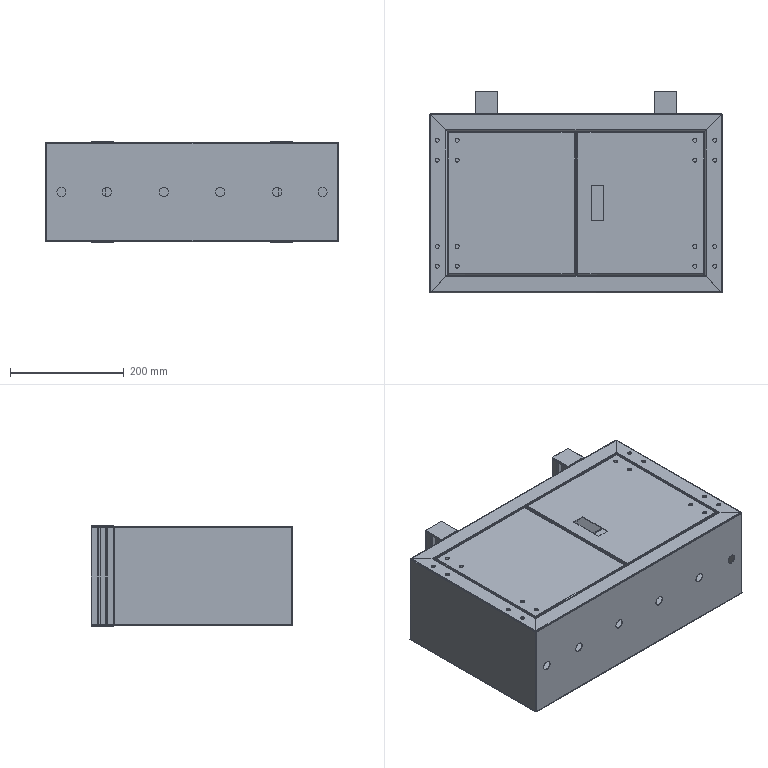Part | 13 solids | 1058 faces | box 515 x 355 x 177 mm | volume 981758 mm3 | plane 634 | cylinder 262 | cone 96 | spline 62 | torus 4 | commonest cylinder face diameters 1.5 x64 1.473 x32 3.873 x32 7 x32 4 x16 2.2 x12